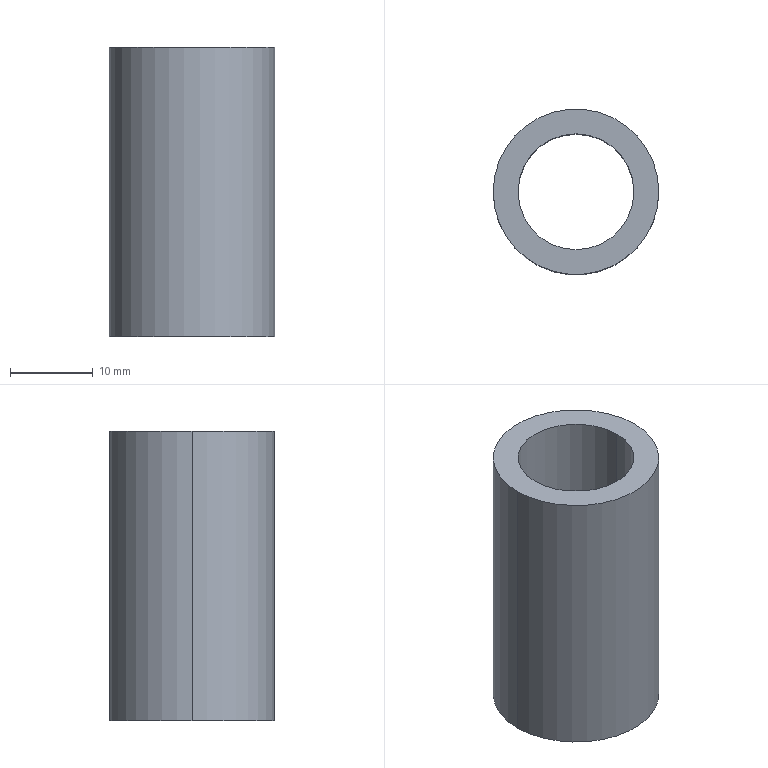Part | SolidWorks | features Extrusion 1 | 1 solid | 6 faces | box 20 x 20 x 35 mm | volume 5608 mm3 | cylinder 4 | plane 2 | commonest cylinder face diameters 14 x2 20 x2
STEP:
#1=CARTESIAN_POINT('',(-7.,0.,35.));
#2=VERTEX_POINT('',#1);
#3=CARTESIAN_POINT('',(7.,0.,35.));
#4=VERTEX_POINT('',#3);
#5=CARTESIAN_POINT('',(0.,0.,35.));
#6=DIRECTION('',(0.,0.,1.));
#7=DIRECTION('',(1.,0.,0.));
#8=AXIS2_PLACEMENT_3D('',#5,#6,#7);
#9=CIRCLE('',#8,7.);
#10=EDGE_CURVE('',#2,#4,#9,.T.);
#11=ORIENTED_EDGE('',*,*,#10,.T.);
#12=CARTESIAN_POINT('',(7.,0.,0.));
#13=VERTEX_POINT('',#12);
#14=CARTESIAN_POINT('',(7.,0.,35.));
#15=DIRECTION('',(0.,0.,-1.));
#16=VECTOR('',#15,1000.);
#17=LINE('',#14,#16);
#18=EDGE_CURVE('',#4,#13,#17,.T.);
#19=ORIENTED_EDGE('',*,*,#18,.T.);
#20=CARTESIAN_POINT('',(-7.,0.,0.));
#21=VERTEX_POINT('',#20);
#22=CARTESIAN_POINT('',(0.,0.,0.));
#23=DIRECTION('',(0.,0.,1.));
#24=DIRECTION('',(1.,0.,0.));
#25=AXIS2_PLACEMENT_3D('',#22,#23,#24);
#26=CIRCLE('',#25,7.);
#27=EDGE_CURVE('',#21,#13,#26,.T.);
#28=ORIENTED_EDGE('',*,*,#27,.F.);
#29=CARTESIAN_POINT('',(-7.,0.,35.));
#30=DIRECTION('',(0.,0.,-1.));
#31=VECTOR('',#30,1000.);
#32=LINE('',#29,#31);
#33=EDGE_CURVE('',#2,#21,#32,.T.);
#34=ORIENTED_EDGE('',*,*,#33,.F.);
#35=EDGE_LOOP('',(#11,#19,#28,#34));
#36=FACE_OUTER_BOUND('',#35,.T.);
#37=CARTESIAN_POINT('',(0.,0.,35.));
#38=DIRECTION('',(0.,0.,-1.));
#39=DIRECTION('',(-1.,0.,0.));
#40=AXIS2_PLACEMENT_3D('',#37,#38,#39);
#41=CYLINDRICAL_SURFACE('',#40,7.);
#42=ADVANCED_FACE('',(#36),#41,.F.);
#43=CARTESIAN_POINT('',(10.,0.,35.));
#44=VERTEX_POINT('',#43);
#45=CARTESIAN_POINT('',(-10.,0.,35.));
#46=VERTEX_POINT('',#45);
#47=CARTESIAN_POINT('',(0.,0.,35.));
#48=DIRECTION('',(0.,0.,1.));
#49=DIRECTION('',(1.,0.,0.));
#50=AXIS2_PLACEMENT_3D('',#47,#48,#49);
#51=CIRCLE('',#50,10.);
#52=EDGE_CURVE('',#44,#46,#51,.T.);
#53=ORIENTED_EDGE('',*,*,#52,.F.);
#54=CARTESIAN_POINT('',(10.,0.,0.));
#55=VERTEX_POINT('',#54);
#56=CARTESIAN_POINT('',(10.,0.,35.));
#57=DIRECTION('',(0.,0.,-1.));
#58=VECTOR('',#57,1000.);
#59=LINE('',#56,#58);
#60=EDGE_CURVE('',#44,#55,#59,.T.);
#61=ORIENTED_EDGE('',*,*,#60,.T.);
#62=CARTESIAN_POINT('',(-10.,0.,0.));
#63=VERTEX_POINT('',#62);
#64=CARTESIAN_POINT('',(0.,0.,0.));
#65=DIRECTION('',(0.,0.,1.));
#66=DIRECTION('',(1.,0.,0.));
#67=AXIS2_PLACEMENT_3D('',#64,#65,#66);
#68=CIRCLE('',#67,10.);
#69=EDGE_CURVE('',#55,#63,#68,.T.);
#70=ORIENTED_EDGE('',*,*,#69,.T.);
#71=CARTESIAN_POINT('',(-10.,0.,35.));
#72=DIRECTION('',(0.,0.,-1.));
#73=VECTOR('',#72,1000.);
#74=LINE('',#71,#73);
#75=EDGE_CURVE('',#46,#63,#74,.T.);
#76=ORIENTED_EDGE('',*,*,#75,.F.);
#77=EDGE_LOOP('',(#53,#61,#70,#76));
#78=FACE_OUTER_BOUND('',#77,.T.);
#79=CARTESIAN_POINT('',(0.,0.,35.));
#80=DIRECTION('',(0.,0.,-1.));
#81=DIRECTION('',(-1.,0.,0.));
#82=AXIS2_PLACEMENT_3D('',#79,#80,#81);
#83=CYLINDRICAL_SURFACE('',#82,10.);
#84=ADVANCED_FACE('',(#78),#83,.T.);
#85=CARTESIAN_POINT('',(0.,0.,35.));
#86=DIRECTION('',(0.,0.,1.));
#87=DIRECTION('',(1.,0.,0.));
#88=AXIS2_PLACEMENT_3D('',#85,#86,#87);
#89=CIRCLE('',#88,10.);
#90=EDGE_CURVE('',#46,#44,#89,.T.);
#91=ORIENTED_EDGE('',*,*,#90,.T.);
#92=ORIENTED_EDGE('',*,*,#52,.T.);
#93=EDGE_LOOP('',(#91,#92));
#94=FACE_OUTER_BOUND('',#93,.T.);
#95=ORIENTED_EDGE('',*,*,#10,.F.);
#96=CARTESIAN_POINT('',(0.,0.,35.));
#97=DIRECTION('',(0.,0.,1.));
#98=DIRECTION('',(1.,0.,0.));
#99=AXIS2_PLACEMENT_3D('',#96,#97,#98);
#100=CIRCLE('',#99,7.);
#101=EDGE_CURVE('',#4,#2,#100,.T.);
#102=ORIENTED_EDGE('',*,*,#101,.F.);
#103=EDGE_LOOP('',(#95,#102));
#104=FACE_BOUND('',#103,.T.);
#105=CARTESIAN_POINT('',(0.,0.,35.));
#106=DIRECTION('',(0.,0.,1.));
#107=DIRECTION('',(1.,0.,0.));
#108=AXIS2_PLACEMENT_3D('',#105,#106,#107);
#109=PLANE('',#108);
#110=ADVANCED_FACE('',(#94,#104),#109,.T.);
#111=CARTESIAN_POINT('',(0.,0.,0.));
#112=DIRECTION('',(0.,0.,1.));
#113=DIRECTION('',(1.,0.,0.));
#114=AXIS2_PLACEMENT_3D('',#111,#112,#113);
#115=CIRCLE('',#114,10.);
#116=EDGE_CURVE('',#63,#55,#115,.T.);
#117=ORIENTED_EDGE('',*,*,#116,.F.);
#118=ORIENTED_EDGE('',*,*,#69,.F.);
#119=EDGE_LOOP('',(#117,#118));
#120=FACE_OUTER_BOUND('',#119,.T.);
#121=ORIENTED_EDGE('',*,*,#27,.T.);
#122=CARTESIAN_POINT('',(0.,0.,0.));
#123=DIRECTION('',(0.,0.,1.));
#124=DIRECTION('',(1.,0.,0.));
#125=AXIS2_PLACEMENT_3D('',#122,#123,#124);
#126=CIRCLE('',#125,7.);
#127=EDGE_CURVE('',#13,#21,#126,.T.);
#128=ORIENTED_EDGE('',*,*,#127,.T.);
#129=EDGE_LOOP('',(#121,#128));
#130=FACE_BOUND('',#129,.T.);
#131=CARTESIAN_POINT('',(0.,0.,0.));
#132=DIRECTION('',(0.,0.,1.));
#133=DIRECTION('',(1.,0.,0.));
#134=AXIS2_PLACEMENT_3D('',#131,#132,#133);
#135=PLANE('',#134);
#136=ADVANCED_FACE('',(#120,#130),#135,.F.);
#137=ORIENTED_EDGE('',*,*,#60,.F.);
#138=ORIENTED_EDGE('',*,*,#90,.F.);
#139=ORIENTED_EDGE('',*,*,#75,.T.);
#140=ORIENTED_EDGE('',*,*,#116,.T.);
#141=EDGE_LOOP('',(#137,#138,#139,#140));
#142=FACE_OUTER_BOUND('',#141,.T.);
#143=CARTESIAN_POINT('',(0.,0.,35.));
#144=DIRECTION('',(0.,0.,-1.));
#145=DIRECTION('',(-1.,0.,0.));
#146=AXIS2_PLACEMENT_3D('',#143,#144,#145);
#147=CYLINDRICAL_SURFACE('',#146,10.);
#148=ADVANCED_FACE('',(#142),#147,.T.);
#149=ORIENTED_EDGE('',*,*,#18,.F.);
#150=ORIENTED_EDGE('',*,*,#101,.T.);
#151=ORIENTED_EDGE('',*,*,#33,.T.);
#152=ORIENTED_EDGE('',*,*,#127,.F.);
#153=EDGE_LOOP('',(#149,#150,#151,#152));
#154=FACE_OUTER_BOUND('',#153,.T.);
#155=CARTESIAN_POINT('',(0.,0.,35.));
#156=DIRECTION('',(0.,0.,-1.));
#157=DIRECTION('',(-1.,0.,0.));
#158=AXIS2_PLACEMENT_3D('',#155,#156,#157);
#159=CYLINDRICAL_SURFACE('',#158,7.);
#160=ADVANCED_FACE('',(#154),#159,.F.);
#161=CLOSED_SHELL('',(#42,#84,#110,#136,#148,#160));
#162=MANIFOLD_SOLID_BREP('',#161);
#163=CARTESIAN_POINT('',(0.,0.,0.));
#164=DIRECTION('',(0.,0.,1.));
#165=DIRECTION('',(1.,0.,0.));
#166=AXIS2_PLACEMENT_3D('',#163,#164,#165);
#167=(LENGTH_UNIT()NAMED_UNIT(*)SI_UNIT(.MILLI.,.METRE.));
#168=UNCERTAINTY_MEASURE_WITH_UNIT(LENGTH_MEASURE(0.00001),#167,'','');
#169=(NAMED_UNIT(*)PLANE_ANGLE_UNIT()SI_UNIT($,.RADIAN.));
#170=(NAMED_UNIT(*)SI_UNIT($,.STERADIAN.)SOLID_ANGLE_UNIT());
#171=(GEOMETRIC_REPRESENTATION_CONTEXT(3)GLOBAL_UNCERTAINTY_ASSIGNED_CONTEXT((#168))GLOBAL_UNIT_ASSIGNED_CONTEXT((#167,#169,#170))REPRESENTATION_CONTEXT('',''));
#172=ADVANCED_BREP_SHAPE_REPRESENTATION('',(#162,#166),#171);